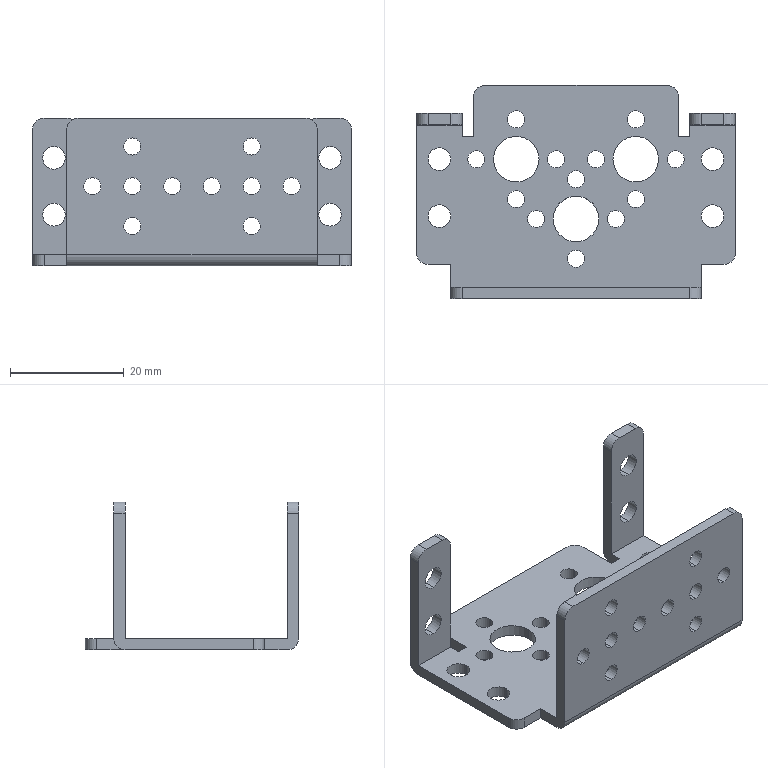Part | SolidWorks | features ICE 8, LPattern 2, Extrusion 1, Fillet 1, MirrorPattern 1 | 1 solid | 103 faces | box 56 x 37.49 x 26 mm | volume 5821 mm3 | cylinder 79 | plane 24 | commonest cylinder face diameters 3 x44 4 x29 8 x6